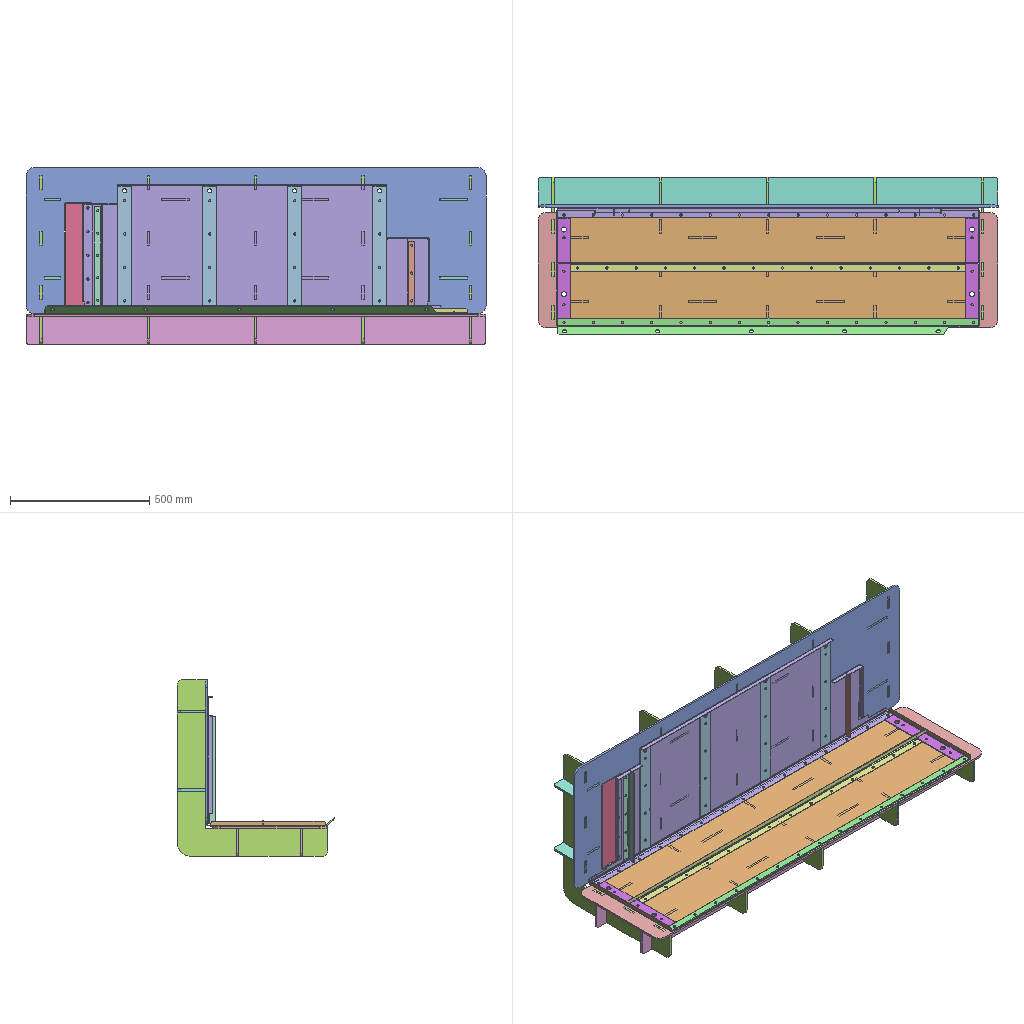Assembly | SolidWorks | 15 different items | 25 placed | box 1650 x 565 x 635 mm
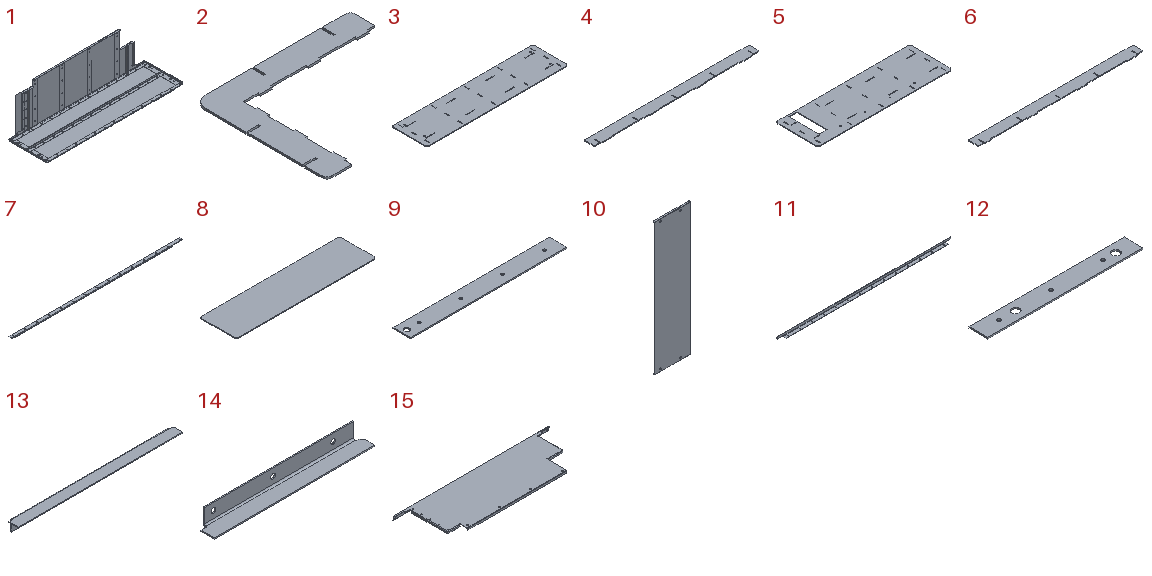Parts list (item | name | quantity | parent item | size | volume | features):
1 | (subassembly) | x1 | - | 1520 x 459.004 x 465.1 mm | 3224415 mm3 | features ReferencePattern 3, CompositeCurve 1, LocalLPattern 1
2 | - | x5 | - | 634.6 x 540 x 8 mm | 859257 mm3 | features FlatPattern 1, SMBaseFlange 1, SheetMetal 1
3 | - | x1 | - | 1650 x 415 x 8 mm | 5364476 mm3 | features FlatPattern 1, SMBaseFlange 1, SheetMetal 1
4 | - | x2 | - | 1650 x 107.5 x 8 mm | 1327497 mm3 | features FlatPattern 1, SMBaseFlange 1, SheetMetal 1
5 | - | x1 | - | 1650 x 525 x 8 mm | 6516839 mm3 | features FlatPattern 1, SMBaseFlange 1, SheetMetal 1
6 | - | x2 | - | 1650 x 107.5 x 8 mm | 1325097 mm3 | features FlatPattern 1, SMBaseFlange 1, SheetMetal 1
7 | - | x1 | in 1 | 1508 x 59.004 x 28.421 mm | 304749 mm3 | features FlatPattern 1, SM3dBend 1, SMBaseFlange 1, SheetMetal 1
8 | - | x1 | in 1 | 372 x 97 x 2 mm | 72125 mm3 | features FlatPattern 1, SMBaseFlange 1, SheetMetal 1
9 | - | x4 | in 1 | 449.5 x 50 x 3.2 mm | 70711 mm3 | features FlatPattern 1, SMBaseFlange 1, SheetMetal 1
10 | - | x1 | in 1 | 413 x 18 x 1520 mm | 1023020 mm3 | features Fillet 1, FlatPattern 1, ICE 1, SMBaseFlange 1, SheetMetal 1
11 | - | x1 | in 1 | 1515 x 30 x 20 mm | 133571 mm3 | features ICE 2, Chamfer 1, FlatPattern 1, SMBaseFlange 1, SheetMetal 1
12 | - | x2 | in 1 | 359 x 44 x 3.2 mm | 48436 mm3 | features FlatPattern 1, SMBaseFlange 1, SheetMetal 1
13 | - | x1 | in 1 | 391.9 x 28 x 28 mm | 39440 mm3 | features ICE 2, Chamfer 1, Fillet 1, FlatPattern 1, SMBaseFlange 1, SheetMetal 1
14 | - | x1 | in 1 | 268.9 x 28 x 28 mm | 26727 mm3 | features ICE 2, Chamfer 1, Fillet 1, FlatPattern 1, SMBaseFlange 1, SheetMetal 1
15 | - | x1 | in 1 | 1508 x 463.5 x 37 mm | 1245074 mm3 | features EdgeFlange 2, CornerRelief 1, Fillet 1, FlatPattern 1, ICE 1, SMBaseFlange 1, SheetMetal 1
Mates (type | each side: item.copy, entity, surface, feature):
In the top assembly
InPlace | 2.1 plane | assembly plane
InPlace | 4.1 plane | assembly plane
InPlace | 6.1 plane | assembly plane
Coincident | 3.1 face plane Base-Flange1 | 10.1 face plane Base-Flange1
Concentric | 3.1 face cylinder Base-Flange1 | 12.1 face cylinder Base-Flange1
Concentric | 3.1 face cylinder Base-Flange1 | 12.2 face cylinder Base-Flange1
In subassembly 1
Coincident | 10.2 face plane Base-Flange1 | 15.1 face plane Edge-Flange1
DistanceDim | 15.1 face plane Base-Flange1 | 10.2 face plane Base-Flange1
DistanceDim | 15.1 face plane Edge-Flange1 | 10.2 face plane Base-Flange1
Coincident | 10.2 face plane Base-Flange1 | 7.1 face plane Base-Flange1
Coincident | 15.1 face plane Edge-Flange1 | 7.1 face plane Base-Flange1
DistanceDim | 7.1 edge | 10.2 face cylinder Cut-Extrude1
DistanceDim | 15.1 face plane Edge-Flange2 | 8.1 face plane Base-Flange1 | 2 times
Coincident | 15.1 face plane Base-Flange1 | 8.1 face plane Base-Flange1
Coincident | 15.1 face plane Base-Flange1 | 9.1 face plane Base-Flange1
Concentric | 15.1 face cylinder Base-Flange1 | 9.1 face cylinder Base-Flange1
Parallel | 15.1 face plane Base-Flange1 | 9.1 face plane Base-Flange1
Coincident | 10.2 face plane Base-Flange1 | 11.1 face plane Base-Flange1
DistanceDim | 10.2 face plane Base-Flange1 | 11.1 face plane Base-Flange1
DistanceDim | 10.2 face cylinder Cut-Extrude1 | 11.1 face plane Base-Flange1
Coincident | 10.2 face plane Base-Flange1 | 12.3 face plane Base-Flange1
Concentric | 10.2 face cylinder Cut-Extrude1 | 12.3 face cylinder Base-Flange1 | 2 times
Coincident | 10.2 face plane Base-Flange1 | 12.4 face plane Base-Flange1
Concentric | 10.2 face cylinder Cut-Extrude1 | 12.4 face cylinder Base-Flange1 | 2 times
Coincident | 15.1 face plane Base-Flange1 | 13.1 face plane Base-Flange1
DistanceDim | 15.1 face plane Edge-Flange1 | 13.1 face plane Base-Flange1
DistanceDim | 13.1 face plane Base-Flange1 | 9.1 face cylinder Base-Flange1
Coincident | 15.1 face plane Base-Flange1 | 14.1 face plane Base-Flange1
DistanceDim | 15.1 face plane Edge-Flange1 | 14.1 face plane Base-Flange1
DistanceDim | 9.2 face cylinder Base-Flange1 | 14.1 face plane Base-Flange1